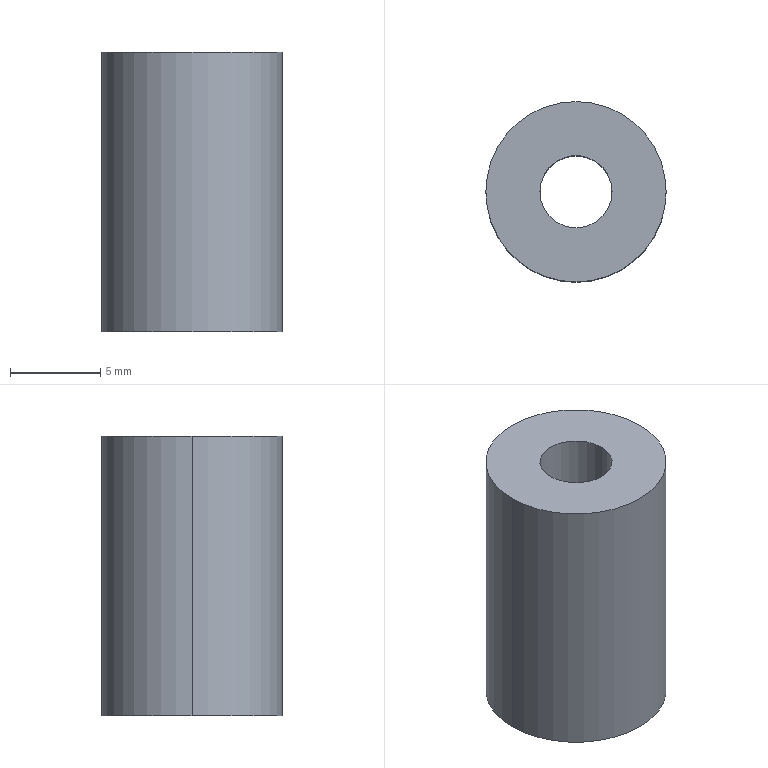Part | SolidWorks | features Extrusion 1 | 1 solid | 6 faces | box 10 x 10 x 15.5 mm | volume 1023 mm3 | cylinder 4 | plane 2 | commonest cylinder face diameters 4 x2 10 x2
STEP:
#1=CARTESIAN_POINT('',(-2.,0.,15.5));
#2=VERTEX_POINT('',#1);
#3=CARTESIAN_POINT('',(2.,0.,15.5));
#4=VERTEX_POINT('',#3);
#5=CARTESIAN_POINT('',(0.,0.,15.5));
#6=DIRECTION('',(0.,0.,1.));
#7=DIRECTION('',(1.,0.,0.));
#8=AXIS2_PLACEMENT_3D('',#5,#6,#7);
#9=CIRCLE('',#8,2.);
#10=EDGE_CURVE('',#2,#4,#9,.T.);
#11=ORIENTED_EDGE('',*,*,#10,.T.);
#12=CARTESIAN_POINT('',(2.,0.,0.));
#13=VERTEX_POINT('',#12);
#14=CARTESIAN_POINT('',(2.,0.,15.5));
#15=DIRECTION('',(0.,0.,-1.));
#16=VECTOR('',#15,1000.);
#17=LINE('',#14,#16);
#18=EDGE_CURVE('',#4,#13,#17,.T.);
#19=ORIENTED_EDGE('',*,*,#18,.T.);
#20=CARTESIAN_POINT('',(-2.,0.,0.));
#21=VERTEX_POINT('',#20);
#22=CARTESIAN_POINT('',(0.,0.,0.));
#23=DIRECTION('',(0.,0.,1.));
#24=DIRECTION('',(1.,0.,0.));
#25=AXIS2_PLACEMENT_3D('',#22,#23,#24);
#26=CIRCLE('',#25,2.);
#27=EDGE_CURVE('',#21,#13,#26,.T.);
#28=ORIENTED_EDGE('',*,*,#27,.F.);
#29=CARTESIAN_POINT('',(-2.,0.,15.5));
#30=DIRECTION('',(0.,0.,-1.));
#31=VECTOR('',#30,1000.);
#32=LINE('',#29,#31);
#33=EDGE_CURVE('',#2,#21,#32,.T.);
#34=ORIENTED_EDGE('',*,*,#33,.F.);
#35=EDGE_LOOP('',(#11,#19,#28,#34));
#36=FACE_OUTER_BOUND('',#35,.T.);
#37=CARTESIAN_POINT('',(0.,0.,15.5));
#38=DIRECTION('',(0.,0.,-1.));
#39=DIRECTION('',(-1.,0.,0.));
#40=AXIS2_PLACEMENT_3D('',#37,#38,#39);
#41=CYLINDRICAL_SURFACE('',#40,2.);
#42=ADVANCED_FACE('',(#36),#41,.F.);
#43=CARTESIAN_POINT('',(5.,0.,15.5));
#44=VERTEX_POINT('',#43);
#45=CARTESIAN_POINT('',(-5.,0.,15.5));
#46=VERTEX_POINT('',#45);
#47=CARTESIAN_POINT('',(0.,0.,15.5));
#48=DIRECTION('',(0.,0.,1.));
#49=DIRECTION('',(1.,0.,0.));
#50=AXIS2_PLACEMENT_3D('',#47,#48,#49);
#51=CIRCLE('',#50,5.);
#52=EDGE_CURVE('',#44,#46,#51,.T.);
#53=ORIENTED_EDGE('',*,*,#52,.F.);
#54=CARTESIAN_POINT('',(5.,0.,0.));
#55=VERTEX_POINT('',#54);
#56=CARTESIAN_POINT('',(5.,0.,15.5));
#57=DIRECTION('',(0.,0.,-1.));
#58=VECTOR('',#57,1000.);
#59=LINE('',#56,#58);
#60=EDGE_CURVE('',#44,#55,#59,.T.);
#61=ORIENTED_EDGE('',*,*,#60,.T.);
#62=CARTESIAN_POINT('',(-5.,0.,0.));
#63=VERTEX_POINT('',#62);
#64=CARTESIAN_POINT('',(0.,0.,0.));
#65=DIRECTION('',(0.,0.,1.));
#66=DIRECTION('',(1.,0.,0.));
#67=AXIS2_PLACEMENT_3D('',#64,#65,#66);
#68=CIRCLE('',#67,5.);
#69=EDGE_CURVE('',#55,#63,#68,.T.);
#70=ORIENTED_EDGE('',*,*,#69,.T.);
#71=CARTESIAN_POINT('',(-5.,0.,15.5));
#72=DIRECTION('',(0.,0.,-1.));
#73=VECTOR('',#72,1000.);
#74=LINE('',#71,#73);
#75=EDGE_CURVE('',#46,#63,#74,.T.);
#76=ORIENTED_EDGE('',*,*,#75,.F.);
#77=EDGE_LOOP('',(#53,#61,#70,#76));
#78=FACE_OUTER_BOUND('',#77,.T.);
#79=CARTESIAN_POINT('',(0.,0.,15.5));
#80=DIRECTION('',(0.,0.,-1.));
#81=DIRECTION('',(-1.,0.,0.));
#82=AXIS2_PLACEMENT_3D('',#79,#80,#81);
#83=CYLINDRICAL_SURFACE('',#82,5.);
#84=ADVANCED_FACE('',(#78),#83,.T.);
#85=CARTESIAN_POINT('',(0.,0.,15.5));
#86=DIRECTION('',(0.,0.,1.));
#87=DIRECTION('',(1.,0.,0.));
#88=AXIS2_PLACEMENT_3D('',#85,#86,#87);
#89=CIRCLE('',#88,5.);
#90=EDGE_CURVE('',#46,#44,#89,.T.);
#91=ORIENTED_EDGE('',*,*,#90,.T.);
#92=ORIENTED_EDGE('',*,*,#52,.T.);
#93=EDGE_LOOP('',(#91,#92));
#94=FACE_OUTER_BOUND('',#93,.T.);
#95=ORIENTED_EDGE('',*,*,#10,.F.);
#96=CARTESIAN_POINT('',(0.,0.,15.5));
#97=DIRECTION('',(0.,0.,1.));
#98=DIRECTION('',(1.,0.,0.));
#99=AXIS2_PLACEMENT_3D('',#96,#97,#98);
#100=CIRCLE('',#99,2.);
#101=EDGE_CURVE('',#4,#2,#100,.T.);
#102=ORIENTED_EDGE('',*,*,#101,.F.);
#103=EDGE_LOOP('',(#95,#102));
#104=FACE_BOUND('',#103,.T.);
#105=CARTESIAN_POINT('',(0.,0.,15.5));
#106=DIRECTION('',(0.,0.,1.));
#107=DIRECTION('',(1.,0.,0.));
#108=AXIS2_PLACEMENT_3D('',#105,#106,#107);
#109=PLANE('',#108);
#110=ADVANCED_FACE('',(#94,#104),#109,.T.);
#111=CARTESIAN_POINT('',(0.,0.,0.));
#112=DIRECTION('',(0.,0.,1.));
#113=DIRECTION('',(1.,0.,0.));
#114=AXIS2_PLACEMENT_3D('',#111,#112,#113);
#115=CIRCLE('',#114,5.);
#116=EDGE_CURVE('',#63,#55,#115,.T.);
#117=ORIENTED_EDGE('',*,*,#116,.F.);
#118=ORIENTED_EDGE('',*,*,#69,.F.);
#119=EDGE_LOOP('',(#117,#118));
#120=FACE_OUTER_BOUND('',#119,.T.);
#121=ORIENTED_EDGE('',*,*,#27,.T.);
#122=CARTESIAN_POINT('',(0.,0.,0.));
#123=DIRECTION('',(0.,0.,1.));
#124=DIRECTION('',(1.,0.,0.));
#125=AXIS2_PLACEMENT_3D('',#122,#123,#124);
#126=CIRCLE('',#125,2.);
#127=EDGE_CURVE('',#13,#21,#126,.T.);
#128=ORIENTED_EDGE('',*,*,#127,.T.);
#129=EDGE_LOOP('',(#121,#128));
#130=FACE_BOUND('',#129,.T.);
#131=CARTESIAN_POINT('',(0.,0.,0.));
#132=DIRECTION('',(0.,0.,1.));
#133=DIRECTION('',(1.,0.,0.));
#134=AXIS2_PLACEMENT_3D('',#131,#132,#133);
#135=PLANE('',#134);
#136=ADVANCED_FACE('',(#120,#130),#135,.F.);
#137=ORIENTED_EDGE('',*,*,#60,.F.);
#138=ORIENTED_EDGE('',*,*,#90,.F.);
#139=ORIENTED_EDGE('',*,*,#75,.T.);
#140=ORIENTED_EDGE('',*,*,#116,.T.);
#141=EDGE_LOOP('',(#137,#138,#139,#140));
#142=FACE_OUTER_BOUND('',#141,.T.);
#143=CARTESIAN_POINT('',(0.,0.,15.5));
#144=DIRECTION('',(0.,0.,-1.));
#145=DIRECTION('',(-1.,0.,0.));
#146=AXIS2_PLACEMENT_3D('',#143,#144,#145);
#147=CYLINDRICAL_SURFACE('',#146,5.);
#148=ADVANCED_FACE('',(#142),#147,.T.);
#149=ORIENTED_EDGE('',*,*,#18,.F.);
#150=ORIENTED_EDGE('',*,*,#101,.T.);
#151=ORIENTED_EDGE('',*,*,#33,.T.);
#152=ORIENTED_EDGE('',*,*,#127,.F.);
#153=EDGE_LOOP('',(#149,#150,#151,#152));
#154=FACE_OUTER_BOUND('',#153,.T.);
#155=CARTESIAN_POINT('',(0.,0.,15.5));
#156=DIRECTION('',(0.,0.,-1.));
#157=DIRECTION('',(-1.,0.,0.));
#158=AXIS2_PLACEMENT_3D('',#155,#156,#157);
#159=CYLINDRICAL_SURFACE('',#158,2.);
#160=ADVANCED_FACE('',(#154),#159,.F.);
#161=CLOSED_SHELL('',(#42,#84,#110,#136,#148,#160));
#162=MANIFOLD_SOLID_BREP('',#161);
#163=CARTESIAN_POINT('',(0.,0.,0.));
#164=DIRECTION('',(0.,0.,1.));
#165=DIRECTION('',(1.,0.,0.));
#166=AXIS2_PLACEMENT_3D('',#163,#164,#165);
#167=(LENGTH_UNIT()NAMED_UNIT(*)SI_UNIT(.MILLI.,.METRE.));
#168=UNCERTAINTY_MEASURE_WITH_UNIT(LENGTH_MEASURE(0.00001),#167,'','');
#169=(NAMED_UNIT(*)PLANE_ANGLE_UNIT()SI_UNIT($,.RADIAN.));
#170=(NAMED_UNIT(*)SI_UNIT($,.STERADIAN.)SOLID_ANGLE_UNIT());
#171=(GEOMETRIC_REPRESENTATION_CONTEXT(3)GLOBAL_UNCERTAINTY_ASSIGNED_CONTEXT((#168))GLOBAL_UNIT_ASSIGNED_CONTEXT((#167,#169,#170))REPRESENTATION_CONTEXT('',''));
#172=ADVANCED_BREP_SHAPE_REPRESENTATION('',(#162,#166),#171);